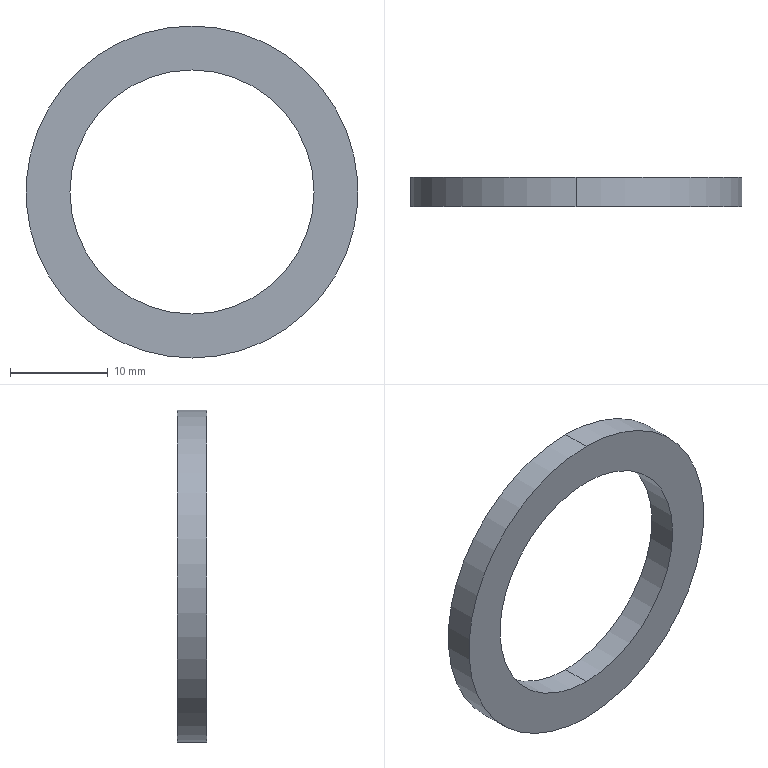Part | SolidWorks | features MirrorStock 1 | 1 solid | 6 faces | box 34 x 3 x 34 mm | volume 1251 mm3 | cylinder 4 | plane 2 | commonest cylinder face diameters 25 x2 34 x2
STEP:
#1=CARTESIAN_POINT('',(0.,1.5,-12.5));
#2=VERTEX_POINT('',#1);
#3=CARTESIAN_POINT('',(0.,1.5,12.5));
#4=VERTEX_POINT('',#3);
#5=CARTESIAN_POINT('',(0.,1.5,0.));
#6=DIRECTION('',(0.,-1.,0.));
#7=DIRECTION('',(0.,0.,-1.));
#8=AXIS2_PLACEMENT_3D('',#5,#6,#7);
#9=CIRCLE('',#8,12.5);
#10=EDGE_CURVE('',#2,#4,#9,.T.);
#11=ORIENTED_EDGE('',*,*,#10,.F.);
#12=CARTESIAN_POINT('',(0.,-1.5,-12.5));
#13=VERTEX_POINT('',#12);
#14=CARTESIAN_POINT('',(0.,1.5,-12.5));
#15=DIRECTION('',(0.,-1.,0.));
#16=VECTOR('',#15,1000.);
#17=LINE('',#14,#16);
#18=EDGE_CURVE('',#2,#13,#17,.T.);
#19=ORIENTED_EDGE('',*,*,#18,.T.);
#20=CARTESIAN_POINT('',(0.,-1.5,12.5));
#21=VERTEX_POINT('',#20);
#22=CARTESIAN_POINT('',(0.,-1.5,0.));
#23=DIRECTION('',(0.,-1.,0.));
#24=DIRECTION('',(0.,0.,-1.));
#25=AXIS2_PLACEMENT_3D('',#22,#23,#24);
#26=CIRCLE('',#25,12.5);
#27=EDGE_CURVE('',#13,#21,#26,.T.);
#28=ORIENTED_EDGE('',*,*,#27,.T.);
#29=CARTESIAN_POINT('',(0.,1.5,12.5));
#30=DIRECTION('',(0.,-1.,0.));
#31=VECTOR('',#30,1000.);
#32=LINE('',#29,#31);
#33=EDGE_CURVE('',#4,#21,#32,.T.);
#34=ORIENTED_EDGE('',*,*,#33,.F.);
#35=EDGE_LOOP('',(#11,#19,#28,#34));
#36=FACE_OUTER_BOUND('',#35,.T.);
#37=CARTESIAN_POINT('',(0.,1.5,0.));
#38=DIRECTION('',(0.,-1.,0.));
#39=DIRECTION('',(0.,0.,1.));
#40=AXIS2_PLACEMENT_3D('',#37,#38,#39);
#41=CYLINDRICAL_SURFACE('',#40,12.5);
#42=ADVANCED_FACE('',(#36),#41,.F.);
#43=CARTESIAN_POINT('',(0.,1.5,17.));
#44=VERTEX_POINT('',#43);
#45=CARTESIAN_POINT('',(0.,1.5,-17.));
#46=VERTEX_POINT('',#45);
#47=CARTESIAN_POINT('',(0.,1.5,0.));
#48=DIRECTION('',(0.,-1.,0.));
#49=DIRECTION('',(0.,0.,-1.));
#50=AXIS2_PLACEMENT_3D('',#47,#48,#49);
#51=CIRCLE('',#50,17.);
#52=EDGE_CURVE('',#44,#46,#51,.T.);
#53=ORIENTED_EDGE('',*,*,#52,.T.);
#54=CARTESIAN_POINT('',(0.,-1.5,-17.));
#55=VERTEX_POINT('',#54);
#56=CARTESIAN_POINT('',(0.,1.5,-17.));
#57=DIRECTION('',(0.,-1.,0.));
#58=VECTOR('',#57,1000.);
#59=LINE('',#56,#58);
#60=EDGE_CURVE('',#46,#55,#59,.T.);
#61=ORIENTED_EDGE('',*,*,#60,.T.);
#62=CARTESIAN_POINT('',(0.,-1.5,17.));
#63=VERTEX_POINT('',#62);
#64=CARTESIAN_POINT('',(0.,-1.5,0.));
#65=DIRECTION('',(0.,-1.,0.));
#66=DIRECTION('',(0.,0.,-1.));
#67=AXIS2_PLACEMENT_3D('',#64,#65,#66);
#68=CIRCLE('',#67,17.);
#69=EDGE_CURVE('',#63,#55,#68,.T.);
#70=ORIENTED_EDGE('',*,*,#69,.F.);
#71=CARTESIAN_POINT('',(0.,1.5,17.));
#72=DIRECTION('',(0.,-1.,0.));
#73=VECTOR('',#72,1000.);
#74=LINE('',#71,#73);
#75=EDGE_CURVE('',#44,#63,#74,.T.);
#76=ORIENTED_EDGE('',*,*,#75,.F.);
#77=EDGE_LOOP('',(#53,#61,#70,#76));
#78=FACE_OUTER_BOUND('',#77,.T.);
#79=CARTESIAN_POINT('',(0.,1.5,0.));
#80=DIRECTION('',(0.,-1.,0.));
#81=DIRECTION('',(0.,0.,1.));
#82=AXIS2_PLACEMENT_3D('',#79,#80,#81);
#83=CYLINDRICAL_SURFACE('',#82,17.);
#84=ADVANCED_FACE('',(#78),#83,.T.);
#85=ORIENTED_EDGE('',*,*,#52,.F.);
#86=CARTESIAN_POINT('',(0.,1.5,0.));
#87=DIRECTION('',(0.,-1.,0.));
#88=DIRECTION('',(0.,0.,-1.));
#89=AXIS2_PLACEMENT_3D('',#86,#87,#88);
#90=CIRCLE('',#89,17.);
#91=EDGE_CURVE('',#46,#44,#90,.T.);
#92=ORIENTED_EDGE('',*,*,#91,.F.);
#93=EDGE_LOOP('',(#85,#92));
#94=FACE_OUTER_BOUND('',#93,.T.);
#95=CARTESIAN_POINT('',(0.,1.5,0.));
#96=DIRECTION('',(0.,-1.,0.));
#97=DIRECTION('',(0.,0.,-1.));
#98=AXIS2_PLACEMENT_3D('',#95,#96,#97);
#99=CIRCLE('',#98,12.5);
#100=EDGE_CURVE('',#4,#2,#99,.T.);
#101=ORIENTED_EDGE('',*,*,#100,.T.);
#102=ORIENTED_EDGE('',*,*,#10,.T.);
#103=EDGE_LOOP('',(#101,#102));
#104=FACE_BOUND('',#103,.T.);
#105=CARTESIAN_POINT('',(0.,1.5,0.));
#106=DIRECTION('',(0.,1.,0.));
#107=DIRECTION('',(0.,0.,-1.));
#108=AXIS2_PLACEMENT_3D('',#105,#106,#107);
#109=PLANE('',#108);
#110=ADVANCED_FACE('',(#94,#104),#109,.T.);
#111=ORIENTED_EDGE('',*,*,#69,.T.);
#112=CARTESIAN_POINT('',(0.,-1.5,0.));
#113=DIRECTION('',(0.,-1.,0.));
#114=DIRECTION('',(0.,0.,-1.));
#115=AXIS2_PLACEMENT_3D('',#112,#113,#114);
#116=CIRCLE('',#115,17.);
#117=EDGE_CURVE('',#55,#63,#116,.T.);
#118=ORIENTED_EDGE('',*,*,#117,.T.);
#119=EDGE_LOOP('',(#111,#118));
#120=FACE_OUTER_BOUND('',#119,.T.);
#121=CARTESIAN_POINT('',(0.,-1.5,0.));
#122=DIRECTION('',(0.,-1.,0.));
#123=DIRECTION('',(0.,0.,-1.));
#124=AXIS2_PLACEMENT_3D('',#121,#122,#123);
#125=CIRCLE('',#124,12.5);
#126=EDGE_CURVE('',#21,#13,#125,.T.);
#127=ORIENTED_EDGE('',*,*,#126,.F.);
#128=ORIENTED_EDGE('',*,*,#27,.F.);
#129=EDGE_LOOP('',(#127,#128));
#130=FACE_BOUND('',#129,.T.);
#131=CARTESIAN_POINT('',(0.,-1.5,0.));
#132=DIRECTION('',(0.,1.,0.));
#133=DIRECTION('',(0.,0.,-1.));
#134=AXIS2_PLACEMENT_3D('',#131,#132,#133);
#135=PLANE('',#134);
#136=ADVANCED_FACE('',(#120,#130),#135,.F.);
#137=ORIENTED_EDGE('',*,*,#60,.F.);
#138=ORIENTED_EDGE('',*,*,#91,.T.);
#139=ORIENTED_EDGE('',*,*,#75,.T.);
#140=ORIENTED_EDGE('',*,*,#117,.F.);
#141=EDGE_LOOP('',(#137,#138,#139,#140));
#142=FACE_OUTER_BOUND('',#141,.T.);
#143=CARTESIAN_POINT('',(0.,1.5,0.));
#144=DIRECTION('',(0.,-1.,0.));
#145=DIRECTION('',(0.,0.,1.));
#146=AXIS2_PLACEMENT_3D('',#143,#144,#145);
#147=CYLINDRICAL_SURFACE('',#146,17.);
#148=ADVANCED_FACE('',(#142),#147,.T.);
#149=ORIENTED_EDGE('',*,*,#18,.F.);
#150=ORIENTED_EDGE('',*,*,#100,.F.);
#151=ORIENTED_EDGE('',*,*,#33,.T.);
#152=ORIENTED_EDGE('',*,*,#126,.T.);
#153=EDGE_LOOP('',(#149,#150,#151,#152));
#154=FACE_OUTER_BOUND('',#153,.T.);
#155=CARTESIAN_POINT('',(0.,1.5,0.));
#156=DIRECTION('',(0.,-1.,0.));
#157=DIRECTION('',(0.,0.,1.));
#158=AXIS2_PLACEMENT_3D('',#155,#156,#157);
#159=CYLINDRICAL_SURFACE('',#158,12.5);
#160=ADVANCED_FACE('',(#154),#159,.F.);
#161=CLOSED_SHELL('',(#42,#84,#110,#136,#148,#160));
#162=MANIFOLD_SOLID_BREP('',#161);
#163=CARTESIAN_POINT('',(0.,0.,0.));
#164=DIRECTION('',(0.,0.,1.));
#165=DIRECTION('',(1.,0.,0.));
#166=AXIS2_PLACEMENT_3D('',#163,#164,#165);
#167=(LENGTH_UNIT()NAMED_UNIT(*)SI_UNIT(.MILLI.,.METRE.));
#168=UNCERTAINTY_MEASURE_WITH_UNIT(LENGTH_MEASURE(0.00001),#167,'','');
#169=(NAMED_UNIT(*)PLANE_ANGLE_UNIT()SI_UNIT($,.RADIAN.));
#170=(NAMED_UNIT(*)SI_UNIT($,.STERADIAN.)SOLID_ANGLE_UNIT());
#171=(GEOMETRIC_REPRESENTATION_CONTEXT(3)GLOBAL_UNCERTAINTY_ASSIGNED_CONTEXT((#168))GLOBAL_UNIT_ASSIGNED_CONTEXT((#167,#169,#170))REPRESENTATION_CONTEXT('',''));
#172=ADVANCED_BREP_SHAPE_REPRESENTATION('',(#162,#166),#171);